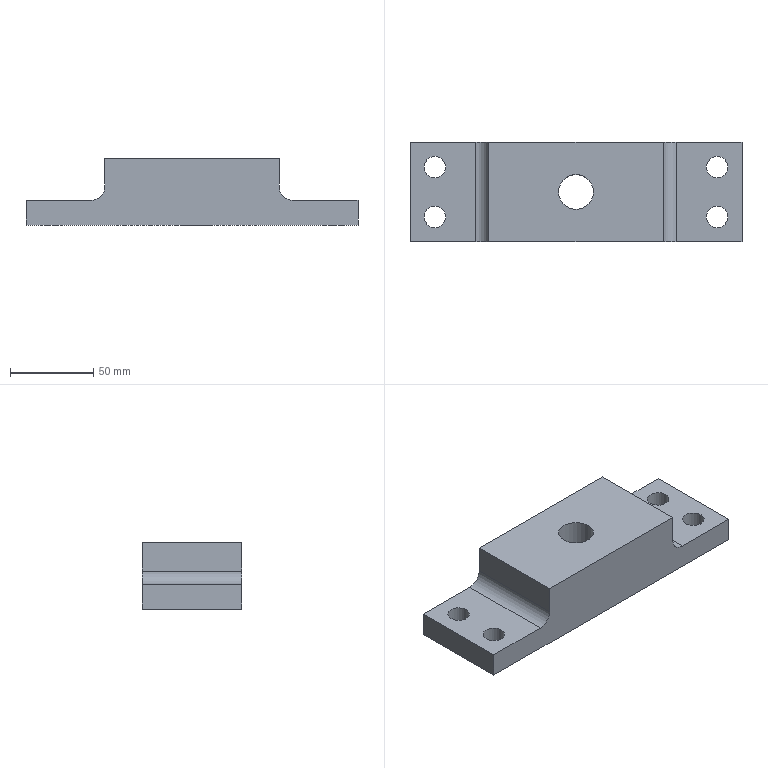Part | NX | features stopper pipe support 2 | 1 solid | 17 faces | box 200 x 60 x 40 mm | volume 317330 mm3 | plane 10 | cylinder 7 | commonest cylinder face diameters 13 x4 16 x2 21 x1
STEP:
#1=CARTESIAN_POINT('',(60.5,-30.,15.));
#2=VERTEX_POINT('',#1);
#3=CARTESIAN_POINT('',(60.5,30.,15.));
#4=VERTEX_POINT('',#3);
#5=CARTESIAN_POINT('',(60.5,30.,15.));
#6=DIRECTION('',(0.,1.,0.));
#7=VECTOR('',#6,1000.);
#8=LINE('',#5,#7);
#9=EDGE_CURVE('',#2,#4,#8,.T.);
#10=ORIENTED_EDGE('',*,*,#9,.T.);
#11=CARTESIAN_POINT('',(52.5,30.,23.));
#12=VERTEX_POINT('',#11);
#13=CARTESIAN_POINT('',(60.5,30.,23.));
#14=DIRECTION('',(0.,-1.,0.));
#15=DIRECTION('',(0.,0.,-1.));
#16=AXIS2_PLACEMENT_3D('',#13,#14,#15);
#17=CIRCLE('',#16,8.);
#18=EDGE_CURVE('',#4,#12,#17,.F.);
#19=ORIENTED_EDGE('',*,*,#18,.T.);
#20=CARTESIAN_POINT('',(52.5,-30.,23.));
#21=VERTEX_POINT('',#20);
#22=CARTESIAN_POINT('',(52.5,-30.,23.));
#23=DIRECTION('',(0.,1.,0.));
#24=VECTOR('',#23,1000.);
#25=LINE('',#22,#24);
#26=EDGE_CURVE('',#12,#21,#25,.F.);
#27=ORIENTED_EDGE('',*,*,#26,.T.);
#28=CARTESIAN_POINT('',(60.5,-30.,23.));
#29=DIRECTION('',(0.,-1.,0.));
#30=DIRECTION('',(0.,0.,-1.));
#31=AXIS2_PLACEMENT_3D('',#28,#29,#30);
#32=CIRCLE('',#31,8.);
#33=EDGE_CURVE('',#21,#2,#32,.T.);
#34=ORIENTED_EDGE('',*,*,#33,.T.);
#35=EDGE_LOOP('',(#10,#19,#27,#34));
#36=FACE_BOUND('',#35,.T.);
#37=CARTESIAN_POINT('',(60.5,-30.,23.));
#38=DIRECTION('',(0.,-1.,0.));
#39=DIRECTION('',(0.,0.,-1.));
#40=AXIS2_PLACEMENT_3D('',#37,#38,#39);
#41=CYLINDRICAL_SURFACE('',#40,8.);
#42=ADVANCED_FACE('',(#36),#41,.F.);
#43=ORIENTED_EDGE('',*,*,#26,.F.);
#44=CARTESIAN_POINT('',(52.5,30.,40.));
#45=VERTEX_POINT('',#44);
#46=CARTESIAN_POINT('',(52.5,30.,15.));
#47=DIRECTION('',(0.,0.,-1.));
#48=VECTOR('',#47,1000.);
#49=LINE('',#46,#48);
#50=EDGE_CURVE('',#12,#45,#49,.F.);
#51=ORIENTED_EDGE('',*,*,#50,.T.);
#52=CARTESIAN_POINT('',(52.5,-30.,40.));
#53=VERTEX_POINT('',#52);
#54=CARTESIAN_POINT('',(52.5,30.,40.));
#55=DIRECTION('',(0.,1.,0.));
#56=VECTOR('',#55,1000.);
#57=LINE('',#54,#56);
#58=EDGE_CURVE('',#53,#45,#57,.T.);
#59=ORIENTED_EDGE('',*,*,#58,.F.);
#60=CARTESIAN_POINT('',(52.5,-30.,15.));
#61=DIRECTION('',(0.,0.,1.));
#62=VECTOR('',#61,1000.);
#63=LINE('',#60,#62);
#64=EDGE_CURVE('',#53,#21,#63,.F.);
#65=ORIENTED_EDGE('',*,*,#64,.T.);
#66=EDGE_LOOP('',(#43,#51,#59,#65));
#67=FACE_BOUND('',#66,.T.);
#68=CARTESIAN_POINT('',(52.5,-30.,40.));
#69=DIRECTION('',(-1.,0.,0.));
#70=DIRECTION('',(0.,0.,1.));
#71=AXIS2_PLACEMENT_3D('',#68,#69,#70);
#72=PLANE('',#71);
#73=ADVANCED_FACE('',(#67),#72,.F.);
#74=ORIENTED_EDGE('',*,*,#58,.T.);
#75=CARTESIAN_POINT('',(-52.5,30.,40.));
#76=VERTEX_POINT('',#75);
#77=CARTESIAN_POINT('',(-100.,30.,40.));
#78=DIRECTION('',(1.,0.,0.));
#79=VECTOR('',#78,1000.);
#80=LINE('',#77,#79);
#81=EDGE_CURVE('',#45,#76,#80,.F.);
#82=ORIENTED_EDGE('',*,*,#81,.T.);
#83=CARTESIAN_POINT('',(-52.5,-30.,40.));
#84=VERTEX_POINT('',#83);
#85=CARTESIAN_POINT('',(-52.5,-30.,40.));
#86=DIRECTION('',(0.,1.,0.));
#87=VECTOR('',#86,1000.);
#88=LINE('',#85,#87);
#89=EDGE_CURVE('',#76,#84,#88,.F.);
#90=ORIENTED_EDGE('',*,*,#89,.T.);
#91=CARTESIAN_POINT('',(-100.,-30.,40.));
#92=DIRECTION('',(1.,0.,0.));
#93=VECTOR('',#92,1000.);
#94=LINE('',#91,#93);
#95=EDGE_CURVE('',#84,#53,#94,.T.);
#96=ORIENTED_EDGE('',*,*,#95,.T.);
#97=EDGE_LOOP('',(#74,#82,#90,#96));
#98=FACE_BOUND('',#97,.T.);
#99=CARTESIAN_POINT('',(10.5,0.,40.));
#100=VERTEX_POINT('',#99);
#101=CARTESIAN_POINT('',(0.,0.,40.));
#102=DIRECTION('',(0.,0.,1.));
#103=DIRECTION('',(1.,0.,0.));
#104=AXIS2_PLACEMENT_3D('',#101,#102,#103);
#105=CIRCLE('',#104,10.5);
#106=EDGE_CURVE('',#100,#100,#105,.F.);
#107=ORIENTED_EDGE('',*,*,#106,.T.);
#108=EDGE_LOOP('',(#107));
#109=FACE_BOUND('',#108,.T.);
#110=CARTESIAN_POINT('',(-52.5,30.,40.));
#111=DIRECTION('',(0.,0.,1.));
#112=DIRECTION('',(1.,0.,0.));
#113=AXIS2_PLACEMENT_3D('',#110,#111,#112);
#114=PLANE('',#113);
#115=ADVANCED_FACE('',(#98,#109),#114,.T.);
#116=CARTESIAN_POINT('',(-52.5,30.,23.));
#117=VERTEX_POINT('',#116);
#118=CARTESIAN_POINT('',(-52.5,-30.,23.));
#119=VERTEX_POINT('',#118);
#120=CARTESIAN_POINT('',(-52.5,-30.,23.));
#121=DIRECTION('',(0.,1.,0.));
#122=VECTOR('',#121,1000.);
#123=LINE('',#120,#122);
#124=EDGE_CURVE('',#117,#119,#123,.F.);
#125=ORIENTED_EDGE('',*,*,#124,.T.);
#126=CARTESIAN_POINT('',(-52.5,-30.,15.));
#127=DIRECTION('',(0.,0.,1.));
#128=VECTOR('',#127,1000.);
#129=LINE('',#126,#128);
#130=EDGE_CURVE('',#119,#84,#129,.T.);
#131=ORIENTED_EDGE('',*,*,#130,.T.);
#132=ORIENTED_EDGE('',*,*,#89,.F.);
#133=CARTESIAN_POINT('',(-52.5,30.,15.));
#134=DIRECTION('',(0.,0.,-1.));
#135=VECTOR('',#134,1000.);
#136=LINE('',#133,#135);
#137=EDGE_CURVE('',#76,#117,#136,.T.);
#138=ORIENTED_EDGE('',*,*,#137,.T.);
#139=EDGE_LOOP('',(#125,#131,#132,#138));
#140=FACE_BOUND('',#139,.T.);
#141=CARTESIAN_POINT('',(-52.5,-30.,40.));
#142=DIRECTION('',(1.,0.,0.));
#143=DIRECTION('',(0.,0.,-1.));
#144=AXIS2_PLACEMENT_3D('',#141,#142,#143);
#145=PLANE('',#144);
#146=ADVANCED_FACE('',(#140),#145,.F.);
#147=CARTESIAN_POINT('',(-60.5,30.,15.));
#148=VERTEX_POINT('',#147);
#149=CARTESIAN_POINT('',(-60.5,-30.,15.));
#150=VERTEX_POINT('',#149);
#151=CARTESIAN_POINT('',(-60.5,30.,15.));
#152=DIRECTION('',(0.,1.,0.));
#153=VECTOR('',#152,1000.);
#154=LINE('',#151,#153);
#155=EDGE_CURVE('',#148,#150,#154,.F.);
#156=ORIENTED_EDGE('',*,*,#155,.T.);
#157=CARTESIAN_POINT('',(-60.5,-30.,23.));
#158=DIRECTION('',(0.,1.,0.));
#159=DIRECTION('',(0.,0.,1.));
#160=AXIS2_PLACEMENT_3D('',#157,#158,#159);
#161=CIRCLE('',#160,8.);
#162=EDGE_CURVE('',#150,#119,#161,.F.);
#163=ORIENTED_EDGE('',*,*,#162,.T.);
#164=ORIENTED_EDGE('',*,*,#124,.F.);
#165=CARTESIAN_POINT('',(-60.5,30.,23.));
#166=DIRECTION('',(0.,1.,0.));
#167=DIRECTION('',(0.,0.,1.));
#168=AXIS2_PLACEMENT_3D('',#165,#166,#167);
#169=CIRCLE('',#168,8.);
#170=EDGE_CURVE('',#117,#148,#169,.T.);
#171=ORIENTED_EDGE('',*,*,#170,.T.);
#172=EDGE_LOOP('',(#156,#163,#164,#171));
#173=FACE_BOUND('',#172,.T.);
#174=CARTESIAN_POINT('',(-60.5,-30.,23.));
#175=DIRECTION('',(0.,1.,0.));
#176=DIRECTION('',(0.,0.,1.));
#177=AXIS2_PLACEMENT_3D('',#174,#175,#176);
#178=CYLINDRICAL_SURFACE('',#177,8.);
#179=ADVANCED_FACE('',(#173),#178,.F.);
#180=ORIENTED_EDGE('',*,*,#9,.F.);
#181=CARTESIAN_POINT('',(100.,-30.,15.));
#182=VERTEX_POINT('',#181);
#183=CARTESIAN_POINT('',(-100.,-30.,15.));
#184=DIRECTION('',(1.,0.,0.));
#185=VECTOR('',#184,1000.);
#186=LINE('',#183,#185);
#187=EDGE_CURVE('',#2,#182,#186,.T.);
#188=ORIENTED_EDGE('',*,*,#187,.T.);
#189=CARTESIAN_POINT('',(100.,30.,15.));
#190=VERTEX_POINT('',#189);
#191=CARTESIAN_POINT('',(100.,-30.,15.));
#192=DIRECTION('',(0.,1.,0.));
#193=VECTOR('',#192,1000.);
#194=LINE('',#191,#193);
#195=EDGE_CURVE('',#182,#190,#194,.T.);
#196=ORIENTED_EDGE('',*,*,#195,.T.);
#197=CARTESIAN_POINT('',(-100.,30.,15.));
#198=DIRECTION('',(1.,0.,0.));
#199=VECTOR('',#198,1000.);
#200=LINE('',#197,#199);
#201=EDGE_CURVE('',#190,#4,#200,.F.);
#202=ORIENTED_EDGE('',*,*,#201,.T.);
#203=EDGE_LOOP('',(#180,#188,#196,#202));
#204=FACE_BOUND('',#203,.T.);
#205=CARTESIAN_POINT('',(78.5,15.,15.));
#206=VERTEX_POINT('',#205);
#207=CARTESIAN_POINT('',(85.,15.,15.));
#208=DIRECTION('',(0.,0.,-1.));
#209=DIRECTION('',(-1.,0.,0.));
#210=AXIS2_PLACEMENT_3D('',#207,#208,#209);
#211=CIRCLE('',#210,6.5);
#212=EDGE_CURVE('',#206,#206,#211,.T.);
#213=ORIENTED_EDGE('',*,*,#212,.T.);
#214=EDGE_LOOP('',(#213));
#215=FACE_BOUND('',#214,.T.);
#216=CARTESIAN_POINT('',(78.5,-15.,15.));
#217=VERTEX_POINT('',#216);
#218=CARTESIAN_POINT('',(85.,-15.,15.));
#219=DIRECTION('',(0.,0.,-1.));
#220=DIRECTION('',(-1.,0.,0.));
#221=AXIS2_PLACEMENT_3D('',#218,#219,#220);
#222=CIRCLE('',#221,6.5);
#223=EDGE_CURVE('',#217,#217,#222,.T.);
#224=ORIENTED_EDGE('',*,*,#223,.T.);
#225=EDGE_LOOP('',(#224));
#226=FACE_BOUND('',#225,.T.);
#227=CARTESIAN_POINT('',(100.,30.,15.));
#228=DIRECTION('',(0.,0.,-1.));
#229=DIRECTION('',(-1.,0.,0.));
#230=AXIS2_PLACEMENT_3D('',#227,#228,#229);
#231=PLANE('',#230);
#232=ADVANCED_FACE('',(#204,#215,#226),#231,.F.);
#233=ORIENTED_EDGE('',*,*,#155,.F.);
#234=CARTESIAN_POINT('',(-100.,30.,15.));
#235=VERTEX_POINT('',#234);
#236=CARTESIAN_POINT('',(-100.,30.,15.));
#237=DIRECTION('',(1.,0.,0.));
#238=VECTOR('',#237,1000.);
#239=LINE('',#236,#238);
#240=EDGE_CURVE('',#148,#235,#239,.F.);
#241=ORIENTED_EDGE('',*,*,#240,.T.);
#242=CARTESIAN_POINT('',(-100.,-30.,15.));
#243=VERTEX_POINT('',#242);
#244=CARTESIAN_POINT('',(-100.,-30.,15.));
#245=DIRECTION('',(0.,1.,0.));
#246=VECTOR('',#245,1000.);
#247=LINE('',#244,#246);
#248=EDGE_CURVE('',#235,#243,#247,.F.);
#249=ORIENTED_EDGE('',*,*,#248,.T.);
#250=CARTESIAN_POINT('',(-100.,-30.,15.));
#251=DIRECTION('',(1.,0.,0.));
#252=VECTOR('',#251,1000.);
#253=LINE('',#250,#252);
#254=EDGE_CURVE('',#243,#150,#253,.T.);
#255=ORIENTED_EDGE('',*,*,#254,.T.);
#256=EDGE_LOOP('',(#233,#241,#249,#255));
#257=FACE_BOUND('',#256,.T.);
#258=CARTESIAN_POINT('',(-91.5,-15.,15.));
#259=VERTEX_POINT('',#258);
#260=CARTESIAN_POINT('',(-85.,-15.,15.));
#261=DIRECTION('',(0.,0.,-1.));
#262=DIRECTION('',(-1.,0.,0.));
#263=AXIS2_PLACEMENT_3D('',#260,#261,#262);
#264=CIRCLE('',#263,6.5);
#265=EDGE_CURVE('',#259,#259,#264,.T.);
#266=ORIENTED_EDGE('',*,*,#265,.T.);
#267=EDGE_LOOP('',(#266));
#268=FACE_BOUND('',#267,.T.);
#269=CARTESIAN_POINT('',(-91.5,15.,15.));
#270=VERTEX_POINT('',#269);
#271=CARTESIAN_POINT('',(-85.,15.,15.));
#272=DIRECTION('',(0.,0.,-1.));
#273=DIRECTION('',(-1.,0.,0.));
#274=AXIS2_PLACEMENT_3D('',#271,#272,#273);
#275=CIRCLE('',#274,6.5);
#276=EDGE_CURVE('',#270,#270,#275,.T.);
#277=ORIENTED_EDGE('',*,*,#276,.T.);
#278=EDGE_LOOP('',(#277));
#279=FACE_BOUND('',#278,.T.);
#280=CARTESIAN_POINT('',(100.,30.,15.));
#281=DIRECTION('',(0.,0.,-1.));
#282=DIRECTION('',(-1.,0.,0.));
#283=AXIS2_PLACEMENT_3D('',#280,#281,#282);
#284=PLANE('',#283);
#285=ADVANCED_FACE('',(#257,#268,#279),#284,.F.);
#286=ORIENTED_EDGE('',*,*,#106,.F.);
#287=EDGE_LOOP('',(#286));
#288=FACE_BOUND('',#287,.T.);
#289=CARTESIAN_POINT('',(10.5,0.,0.));
#290=VERTEX_POINT('',#289);
#291=CARTESIAN_POINT('',(0.,0.,0.));
#292=DIRECTION('',(0.,0.,1.));
#293=DIRECTION('',(1.,0.,0.));
#294=AXIS2_PLACEMENT_3D('',#291,#292,#293);
#295=CIRCLE('',#294,10.5);
#296=EDGE_CURVE('',#290,#290,#295,.T.);
#297=ORIENTED_EDGE('',*,*,#296,.F.);
#298=EDGE_LOOP('',(#297));
#299=FACE_BOUND('',#298,.T.);
#300=CARTESIAN_POINT('',(0.,0.,40.));
#301=DIRECTION('',(0.,0.,1.));
#302=DIRECTION('',(1.,0.,0.));
#303=AXIS2_PLACEMENT_3D('',#300,#301,#302);
#304=CYLINDRICAL_SURFACE('',#303,10.5);
#305=ADVANCED_FACE('',(#288,#299),#304,.F.);
#306=ORIENTED_EDGE('',*,*,#265,.F.);
#307=EDGE_LOOP('',(#306));
#308=FACE_BOUND('',#307,.T.);
#309=CARTESIAN_POINT('',(-91.5,-15.,0.));
#310=VERTEX_POINT('',#309);
#311=CARTESIAN_POINT('',(-85.,-15.,0.));
#312=DIRECTION('',(0.,0.,-1.));
#313=DIRECTION('',(-1.,0.,0.));
#314=AXIS2_PLACEMENT_3D('',#311,#312,#313);
#315=CIRCLE('',#314,6.5);
#316=EDGE_CURVE('',#310,#310,#315,.F.);
#317=ORIENTED_EDGE('',*,*,#316,.F.);
#318=EDGE_LOOP('',(#317));
#319=FACE_BOUND('',#318,.T.);
#320=CARTESIAN_POINT('',(-85.,-15.,15.));
#321=DIRECTION('',(0.,0.,-1.));
#322=DIRECTION('',(-1.,0.,0.));
#323=AXIS2_PLACEMENT_3D('',#320,#321,#322);
#324=CYLINDRICAL_SURFACE('',#323,6.5);
#325=ADVANCED_FACE('',(#308,#319),#324,.F.);
#326=ORIENTED_EDGE('',*,*,#212,.F.);
#327=EDGE_LOOP('',(#326));
#328=FACE_BOUND('',#327,.T.);
#329=CARTESIAN_POINT('',(78.5,15.,0.));
#330=VERTEX_POINT('',#329);
#331=CARTESIAN_POINT('',(85.,15.,0.));
#332=DIRECTION('',(0.,0.,-1.));
#333=DIRECTION('',(-1.,0.,0.));
#334=AXIS2_PLACEMENT_3D('',#331,#332,#333);
#335=CIRCLE('',#334,6.5);
#336=EDGE_CURVE('',#330,#330,#335,.F.);
#337=ORIENTED_EDGE('',*,*,#336,.F.);
#338=EDGE_LOOP('',(#337));
#339=FACE_BOUND('',#338,.T.);
#340=CARTESIAN_POINT('',(85.,15.,15.));
#341=DIRECTION('',(0.,0.,-1.));
#342=DIRECTION('',(-1.,0.,0.));
#343=AXIS2_PLACEMENT_3D('',#340,#341,#342);
#344=CYLINDRICAL_SURFACE('',#343,6.5);
#345=ADVANCED_FACE('',(#328,#339),#344,.F.);
#346=CARTESIAN_POINT('',(100.,30.,0.));
#347=VERTEX_POINT('',#346);
#348=CARTESIAN_POINT('',(100.,30.,15.));
#349=DIRECTION('',(0.,0.,-1.));
#350=VECTOR('',#349,1000.);
#351=LINE('',#348,#350);
#352=EDGE_CURVE('',#347,#190,#351,.F.);
#353=ORIENTED_EDGE('',*,*,#352,.T.);
#354=ORIENTED_EDGE('',*,*,#195,.F.);
#355=CARTESIAN_POINT('',(100.,-30.,0.));
#356=VERTEX_POINT('',#355);
#357=CARTESIAN_POINT('',(100.,-30.,15.));
#358=DIRECTION('',(0.,0.,1.));
#359=VECTOR('',#358,1000.);
#360=LINE('',#357,#359);
#361=EDGE_CURVE('',#182,#356,#360,.F.);
#362=ORIENTED_EDGE('',*,*,#361,.T.);
#363=CARTESIAN_POINT('',(100.,30.,0.));
#364=DIRECTION('',(0.,1.,0.));
#365=VECTOR('',#364,1000.);
#366=LINE('',#363,#365);
#367=EDGE_CURVE('',#347,#356,#366,.F.);
#368=ORIENTED_EDGE('',*,*,#367,.F.);
#369=EDGE_LOOP('',(#353,#354,#362,#368));
#370=FACE_BOUND('',#369,.T.);
#371=CARTESIAN_POINT('',(100.,-30.,15.));
#372=DIRECTION('',(-1.,0.,0.));
#373=DIRECTION('',(0.,0.,1.));
#374=AXIS2_PLACEMENT_3D('',#371,#372,#373);
#375=PLANE('',#374);
#376=ADVANCED_FACE('',(#370),#375,.F.);
#377=ORIENTED_EDGE('',*,*,#361,.F.);
#378=ORIENTED_EDGE('',*,*,#187,.F.);
#379=ORIENTED_EDGE('',*,*,#33,.F.);
#380=ORIENTED_EDGE('',*,*,#64,.F.);
#381=ORIENTED_EDGE('',*,*,#95,.F.);
#382=ORIENTED_EDGE('',*,*,#130,.F.);
#383=ORIENTED_EDGE('',*,*,#162,.F.);
#384=ORIENTED_EDGE('',*,*,#254,.F.);
#385=CARTESIAN_POINT('',(-100.,-30.,0.));
#386=VERTEX_POINT('',#385);
#387=CARTESIAN_POINT('',(-100.,-30.,15.));
#388=DIRECTION('',(0.,0.,-1.));
#389=VECTOR('',#388,1000.);
#390=LINE('',#387,#389);
#391=EDGE_CURVE('',#243,#386,#390,.T.);
#392=ORIENTED_EDGE('',*,*,#391,.T.);
#393=CARTESIAN_POINT('',(100.,-30.,0.));
#394=DIRECTION('',(-1.,0.,0.));
#395=VECTOR('',#394,1000.);
#396=LINE('',#393,#395);
#397=EDGE_CURVE('',#356,#386,#396,.T.);
#398=ORIENTED_EDGE('',*,*,#397,.F.);
#399=EDGE_LOOP('',(#377,#378,#379,#380,#381,#382,#383,#384,#392,#398));
#400=FACE_BOUND('',#399,.T.);
#401=CARTESIAN_POINT('',(-100.,-30.,15.));
#402=DIRECTION('',(0.,1.,0.));
#403=DIRECTION('',(0.,0.,1.));
#404=AXIS2_PLACEMENT_3D('',#401,#402,#403);
#405=PLANE('',#404);
#406=ADVANCED_FACE('',(#400),#405,.F.);
#407=ORIENTED_EDGE('',*,*,#391,.F.);
#408=ORIENTED_EDGE('',*,*,#248,.F.);
#409=CARTESIAN_POINT('',(-100.,30.,0.));
#410=VERTEX_POINT('',#409);
#411=CARTESIAN_POINT('',(-100.,30.,15.));
#412=DIRECTION('',(0.,0.,-1.));
#413=VECTOR('',#412,1000.);
#414=LINE('',#411,#413);
#415=EDGE_CURVE('',#235,#410,#414,.T.);
#416=ORIENTED_EDGE('',*,*,#415,.T.);
#417=CARTESIAN_POINT('',(-100.,30.,0.));
#418=DIRECTION('',(0.,1.,0.));
#419=VECTOR('',#418,1000.);
#420=LINE('',#417,#419);
#421=EDGE_CURVE('',#386,#410,#420,.T.);
#422=ORIENTED_EDGE('',*,*,#421,.F.);
#423=EDGE_LOOP('',(#407,#408,#416,#422));
#424=FACE_BOUND('',#423,.T.);
#425=CARTESIAN_POINT('',(-100.,-30.,15.));
#426=DIRECTION('',(1.,0.,0.));
#427=DIRECTION('',(0.,0.,-1.));
#428=AXIS2_PLACEMENT_3D('',#425,#426,#427);
#429=PLANE('',#428);
#430=ADVANCED_FACE('',(#424),#429,.F.);
#431=ORIENTED_EDGE('',*,*,#415,.F.);
#432=ORIENTED_EDGE('',*,*,#240,.F.);
#433=ORIENTED_EDGE('',*,*,#170,.F.);
#434=ORIENTED_EDGE('',*,*,#137,.F.);
#435=ORIENTED_EDGE('',*,*,#81,.F.);
#436=ORIENTED_EDGE('',*,*,#50,.F.);
#437=ORIENTED_EDGE('',*,*,#18,.F.);
#438=ORIENTED_EDGE('',*,*,#201,.F.);
#439=ORIENTED_EDGE('',*,*,#352,.F.);
#440=CARTESIAN_POINT('',(100.,30.,0.));
#441=DIRECTION('',(-1.,0.,0.));
#442=VECTOR('',#441,1000.);
#443=LINE('',#440,#442);
#444=EDGE_CURVE('',#410,#347,#443,.F.);
#445=ORIENTED_EDGE('',*,*,#444,.F.);
#446=EDGE_LOOP('',(#431,#432,#433,#434,#435,#436,#437,#438,#439,#445));
#447=FACE_BOUND('',#446,.T.);
#448=CARTESIAN_POINT('',(-100.,30.,15.));
#449=DIRECTION('',(0.,-1.,0.));
#450=DIRECTION('',(0.,0.,-1.));
#451=AXIS2_PLACEMENT_3D('',#448,#449,#450);
#452=PLANE('',#451);
#453=ADVANCED_FACE('',(#447),#452,.F.);
#454=ORIENTED_EDGE('',*,*,#223,.F.);
#455=EDGE_LOOP('',(#454));
#456=FACE_BOUND('',#455,.T.);
#457=CARTESIAN_POINT('',(78.5,-15.,0.));
#458=VERTEX_POINT('',#457);
#459=CARTESIAN_POINT('',(85.,-15.,0.));
#460=DIRECTION('',(0.,0.,-1.));
#461=DIRECTION('',(-1.,0.,0.));
#462=AXIS2_PLACEMENT_3D('',#459,#460,#461);
#463=CIRCLE('',#462,6.5);
#464=EDGE_CURVE('',#458,#458,#463,.F.);
#465=ORIENTED_EDGE('',*,*,#464,.F.);
#466=EDGE_LOOP('',(#465));
#467=FACE_BOUND('',#466,.T.);
#468=CARTESIAN_POINT('',(85.,-15.,15.));
#469=DIRECTION('',(0.,0.,-1.));
#470=DIRECTION('',(-1.,0.,0.));
#471=AXIS2_PLACEMENT_3D('',#468,#469,#470);
#472=CYLINDRICAL_SURFACE('',#471,6.5);
#473=ADVANCED_FACE('',(#456,#467),#472,.F.);
#474=ORIENTED_EDGE('',*,*,#276,.F.);
#475=EDGE_LOOP('',(#474));
#476=FACE_BOUND('',#475,.T.);
#477=CARTESIAN_POINT('',(-91.5,15.,0.));
#478=VERTEX_POINT('',#477);
#479=CARTESIAN_POINT('',(-85.,15.,0.));
#480=DIRECTION('',(0.,0.,-1.));
#481=DIRECTION('',(-1.,0.,0.));
#482=AXIS2_PLACEMENT_3D('',#479,#480,#481);
#483=CIRCLE('',#482,6.5);
#484=EDGE_CURVE('',#478,#478,#483,.F.);
#485=ORIENTED_EDGE('',*,*,#484,.F.);
#486=EDGE_LOOP('',(#485));
#487=FACE_BOUND('',#486,.T.);
#488=CARTESIAN_POINT('',(-85.,15.,15.));
#489=DIRECTION('',(0.,0.,-1.));
#490=DIRECTION('',(-1.,0.,0.));
#491=AXIS2_PLACEMENT_3D('',#488,#489,#490);
#492=CYLINDRICAL_SURFACE('',#491,6.5);
#493=ADVANCED_FACE('',(#476,#487),#492,.F.);
#494=ORIENTED_EDGE('',*,*,#484,.T.);
#495=EDGE_LOOP('',(#494));
#496=FACE_BOUND('',#495,.T.);
#497=ORIENTED_EDGE('',*,*,#464,.T.);
#498=EDGE_LOOP('',(#497));
#499=FACE_BOUND('',#498,.T.);
#500=ORIENTED_EDGE('',*,*,#421,.T.);
#501=ORIENTED_EDGE('',*,*,#444,.T.);
#502=ORIENTED_EDGE('',*,*,#367,.T.);
#503=ORIENTED_EDGE('',*,*,#397,.T.);
#504=EDGE_LOOP('',(#500,#501,#502,#503));
#505=FACE_BOUND('',#504,.T.);
#506=ORIENTED_EDGE('',*,*,#336,.T.);
#507=EDGE_LOOP('',(#506));
#508=FACE_BOUND('',#507,.T.);
#509=ORIENTED_EDGE('',*,*,#316,.T.);
#510=EDGE_LOOP('',(#509));
#511=FACE_BOUND('',#510,.T.);
#512=ORIENTED_EDGE('',*,*,#296,.T.);
#513=EDGE_LOOP('',(#512));
#514=FACE_BOUND('',#513,.T.);
#515=CARTESIAN_POINT('',(100.,30.,0.));
#516=DIRECTION('',(0.,0.,-1.));
#517=DIRECTION('',(-1.,0.,0.));
#518=AXIS2_PLACEMENT_3D('',#515,#516,#517);
#519=PLANE('',#518);
#520=ADVANCED_FACE('',(#496,#499,#505,#508,#511,#514),#519,.T.);
#521=CLOSED_SHELL('',(#42,#73,#115,#146,#179,#232,#285,#305,#325,#345,#376,#406,#430,#453,#473,#493,#520));
#522=MANIFOLD_SOLID_BREP('',#521);
#523=(LENGTH_UNIT()NAMED_UNIT(*)SI_UNIT(.MILLI.,.METRE.));
#524=UNCERTAINTY_MEASURE_WITH_UNIT(LENGTH_MEASURE(0.00001),#523,'','');
#525=(NAMED_UNIT(*)PLANE_ANGLE_UNIT()SI_UNIT($,.RADIAN.));
#526=(NAMED_UNIT(*)SI_UNIT($,.STERADIAN.)SOLID_ANGLE_UNIT());
#527=(GEOMETRIC_REPRESENTATION_CONTEXT(3)GLOBAL_UNCERTAINTY_ASSIGNED_CONTEXT((#524))GLOBAL_UNIT_ASSIGNED_CONTEXT((#523,#525,#526))REPRESENTATION_CONTEXT('',''));
#528=ADVANCED_BREP_SHAPE_REPRESENTATION('',(#522),#527);